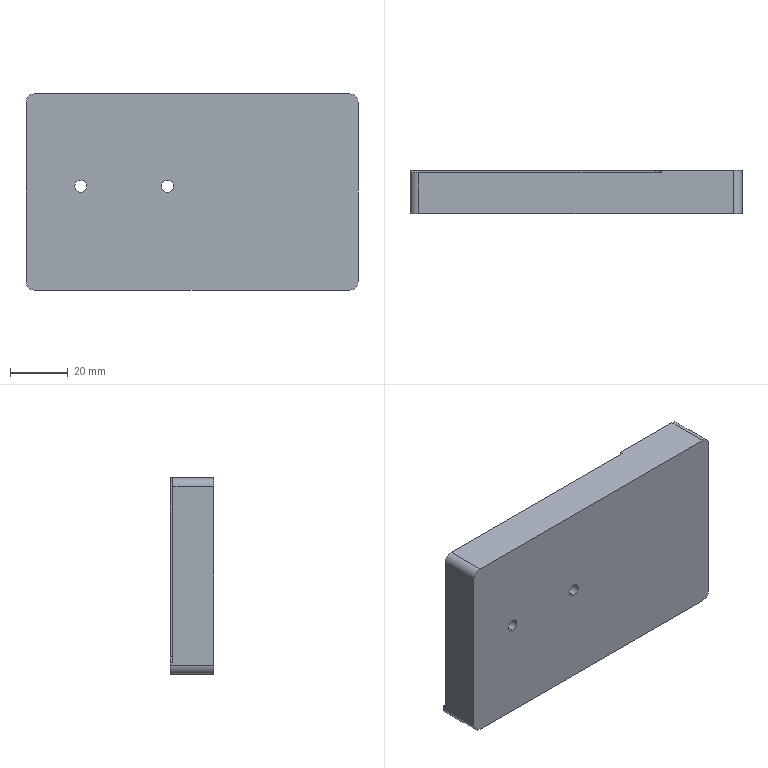Part | STEP file | 10000020445swp000-1 | 1 solid | 26 faces | box 115 x 15 x 68 mm | volume 111374 mm3 | cylinder 13 | plane 9 | cone 4 | commonest cylinder face diameters 4.2 x8 6 x4 4 x1
STEP:
#1=CARTESIAN_POINT('',(7.1,7.5,-19.6));
#2=VERTEX_POINT('',#1);
#3=CARTESIAN_POINT('',(2.9,7.5,-19.6));
#4=VERTEX_POINT('',#3);
#5=CARTESIAN_POINT('',(5.,7.5,-19.6));
#6=DIRECTION('',(0.,0.,-1.));
#7=DIRECTION('',(-1.,0.,0.));
#8=AXIS2_PLACEMENT_3D('',#5,#6,#7);
#9=CIRCLE('',#8,2.1);
#10=EDGE_CURVE('',#2,#4,#9,.T.);
#11=ORIENTED_EDGE('',*,*,#10,.F.);
#12=CARTESIAN_POINT('',(7.1,7.5,-34.));
#13=VERTEX_POINT('',#12);
#14=CARTESIAN_POINT('',(7.1,7.5,-34.));
#15=DIRECTION('',(0.,0.,-1.));
#16=VECTOR('',#15,1000.);
#17=LINE('',#14,#16);
#18=EDGE_CURVE('',#2,#13,#17,.T.);
#19=ORIENTED_EDGE('',*,*,#18,.T.);
#20=CARTESIAN_POINT('',(2.9,7.5,-34.));
#21=VERTEX_POINT('',#20);
#22=CARTESIAN_POINT('',(5.,7.5,-34.));
#23=DIRECTION('',(0.,0.,-1.));
#24=DIRECTION('',(-1.,0.,0.));
#25=AXIS2_PLACEMENT_3D('',#22,#23,#24);
#26=CIRCLE('',#25,2.1);
#27=EDGE_CURVE('',#13,#21,#26,.T.);
#28=ORIENTED_EDGE('',*,*,#27,.T.);
#29=CARTESIAN_POINT('',(2.9,7.5,-34.));
#30=DIRECTION('',(0.,0.,-1.));
#31=VECTOR('',#30,1000.);
#32=LINE('',#29,#31);
#33=EDGE_CURVE('',#4,#21,#32,.T.);
#34=ORIENTED_EDGE('',*,*,#33,.F.);
#35=EDGE_LOOP('',(#11,#19,#28,#34));
#36=FACE_OUTER_BOUND('',#35,.T.);
#37=CARTESIAN_POINT('',(5.,7.5,-34.));
#38=DIRECTION('',(0.,0.,-1.));
#39=DIRECTION('',(-1.,0.,0.));
#40=AXIS2_PLACEMENT_3D('',#37,#38,#39);
#41=CYLINDRICAL_SURFACE('',#40,2.1);
#42=ADVANCED_FACE('',(#36),#41,.F.);
#43=CARTESIAN_POINT('',(5.,7.5,-18.338));
#44=VERTEX_POINT('',#43);
#45=CARTESIAN_POINT('',(2.9,7.5,-19.6));
#46=DIRECTION('',(-0.8572,0.,-0.515));
#47=VECTOR('',#46,1000.);
#48=LINE('',#45,#47);
#49=EDGE_CURVE('',#44,#4,#48,.T.);
#50=ORIENTED_EDGE('',*,*,#49,.F.);
#51=CARTESIAN_POINT('',(7.1,7.5,-19.6));
#52=DIRECTION('',(0.8572,0.,-0.515));
#53=VECTOR('',#52,1000.);
#54=LINE('',#51,#53);
#55=EDGE_CURVE('',#44,#2,#54,.T.);
#56=ORIENTED_EDGE('',*,*,#55,.T.);
#57=ORIENTED_EDGE('',*,*,#10,.T.);
#58=EDGE_LOOP('',(#50,#56,#57));
#59=FACE_OUTER_BOUND('',#58,.T.);
#60=CARTESIAN_POINT('',(5.,7.5,-19.6));
#61=DIRECTION('',(0.,0.,-1.));
#62=DIRECTION('',(-1.,0.,0.));
#63=AXIS2_PLACEMENT_3D('',#60,#61,#62);
#64=CONICAL_SURFACE('',#63,2.1,1.03);
#65=ADVANCED_FACE('',(#59),#64,.F.);
#66=CARTESIAN_POINT('',(-38.9,7.5,-19.6));
#67=VERTEX_POINT('',#66);
#68=CARTESIAN_POINT('',(-43.1,7.5,-19.6));
#69=VERTEX_POINT('',#68);
#70=CARTESIAN_POINT('',(-41.,7.5,-19.6));
#71=DIRECTION('',(0.,0.,-1.));
#72=DIRECTION('',(-1.,0.,0.));
#73=AXIS2_PLACEMENT_3D('',#70,#71,#72);
#74=CIRCLE('',#73,2.1);
#75=EDGE_CURVE('',#67,#69,#74,.T.);
#76=ORIENTED_EDGE('',*,*,#75,.F.);
#77=CARTESIAN_POINT('',(-38.9,7.5,-34.));
#78=VERTEX_POINT('',#77);
#79=CARTESIAN_POINT('',(-38.9,7.5,-34.));
#80=DIRECTION('',(0.,0.,-1.));
#81=VECTOR('',#80,1000.);
#82=LINE('',#79,#81);
#83=EDGE_CURVE('',#67,#78,#82,.T.);
#84=ORIENTED_EDGE('',*,*,#83,.T.);
#85=CARTESIAN_POINT('',(-43.1,7.5,-34.));
#86=VERTEX_POINT('',#85);
#87=CARTESIAN_POINT('',(-41.,7.5,-34.));
#88=DIRECTION('',(0.,0.,-1.));
#89=DIRECTION('',(-1.,0.,0.));
#90=AXIS2_PLACEMENT_3D('',#87,#88,#89);
#91=CIRCLE('',#90,2.1);
#92=EDGE_CURVE('',#78,#86,#91,.T.);
#93=ORIENTED_EDGE('',*,*,#92,.T.);
#94=CARTESIAN_POINT('',(-43.1,7.5,-34.));
#95=DIRECTION('',(0.,0.,-1.));
#96=VECTOR('',#95,1000.);
#97=LINE('',#94,#96);
#98=EDGE_CURVE('',#69,#86,#97,.T.);
#99=ORIENTED_EDGE('',*,*,#98,.F.);
#100=EDGE_LOOP('',(#76,#84,#93,#99));
#101=FACE_OUTER_BOUND('',#100,.T.);
#102=CARTESIAN_POINT('',(-41.,7.5,-34.));
#103=DIRECTION('',(0.,0.,-1.));
#104=DIRECTION('',(-1.,0.,0.));
#105=AXIS2_PLACEMENT_3D('',#102,#103,#104);
#106=CYLINDRICAL_SURFACE('',#105,2.1);
#107=ADVANCED_FACE('',(#101),#106,.F.);
#108=CARTESIAN_POINT('',(-41.,7.5,-18.338));
#109=VERTEX_POINT('',#108);
#110=CARTESIAN_POINT('',(-43.1,7.5,-19.6));
#111=DIRECTION('',(-0.8572,0.,-0.515));
#112=VECTOR('',#111,1000.);
#113=LINE('',#110,#112);
#114=EDGE_CURVE('',#109,#69,#113,.T.);
#115=ORIENTED_EDGE('',*,*,#114,.F.);
#116=CARTESIAN_POINT('',(-38.9,7.5,-19.6));
#117=DIRECTION('',(0.8572,0.,-0.515));
#118=VECTOR('',#117,1000.);
#119=LINE('',#116,#118);
#120=EDGE_CURVE('',#109,#67,#119,.T.);
#121=ORIENTED_EDGE('',*,*,#120,.T.);
#122=ORIENTED_EDGE('',*,*,#75,.T.);
#123=EDGE_LOOP('',(#115,#121,#122));
#124=FACE_OUTER_BOUND('',#123,.T.);
#125=CARTESIAN_POINT('',(-41.,7.5,-19.6));
#126=DIRECTION('',(0.,0.,-1.));
#127=DIRECTION('',(-1.,0.,0.));
#128=AXIS2_PLACEMENT_3D('',#125,#126,#127);
#129=CONICAL_SURFACE('',#128,2.1,1.03);
#130=ADVANCED_FACE('',(#124),#129,.F.);
#131=CARTESIAN_POINT('',(-8.5,0.,-0.1));
#132=VERTEX_POINT('',#131);
#133=CARTESIAN_POINT('',(-8.5,0.,4.1));
#134=VERTEX_POINT('',#133);
#135=CARTESIAN_POINT('',(-8.5,0.,2.));
#136=DIRECTION('',(0.,1.,0.));
#137=DIRECTION('',(0.,0.,1.));
#138=AXIS2_PLACEMENT_3D('',#135,#136,#137);
#139=CIRCLE('',#138,2.1);
#140=EDGE_CURVE('',#132,#134,#139,.T.);
#141=ORIENTED_EDGE('',*,*,#140,.F.);
#142=CARTESIAN_POINT('',(-8.5,14.1,-0.1));
#143=VERTEX_POINT('',#142);
#144=CARTESIAN_POINT('',(-8.5,14.1,-0.1));
#145=DIRECTION('',(0.,1.,0.));
#146=VECTOR('',#145,1000.);
#147=LINE('',#144,#146);
#148=EDGE_CURVE('',#132,#143,#147,.T.);
#149=ORIENTED_EDGE('',*,*,#148,.T.);
#150=CARTESIAN_POINT('',(-8.5,14.1,4.1));
#151=VERTEX_POINT('',#150);
#152=CARTESIAN_POINT('',(-8.5,14.1,2.));
#153=DIRECTION('',(0.,1.,0.));
#154=DIRECTION('',(0.,0.,1.));
#155=AXIS2_PLACEMENT_3D('',#152,#153,#154);
#156=CIRCLE('',#155,2.1);
#157=EDGE_CURVE('',#143,#151,#156,.T.);
#158=ORIENTED_EDGE('',*,*,#157,.T.);
#159=CARTESIAN_POINT('',(-8.5,14.1,4.1));
#160=DIRECTION('',(0.,1.,0.));
#161=VECTOR('',#160,1000.);
#162=LINE('',#159,#161);
#163=EDGE_CURVE('',#134,#151,#162,.T.);
#164=ORIENTED_EDGE('',*,*,#163,.F.);
#165=EDGE_LOOP('',(#141,#149,#158,#164));
#166=FACE_OUTER_BOUND('',#165,.T.);
#167=CARTESIAN_POINT('',(-8.5,14.1,2.));
#168=DIRECTION('',(0.,1.,0.));
#169=DIRECTION('',(0.,0.,1.));
#170=AXIS2_PLACEMENT_3D('',#167,#168,#169);
#171=CYLINDRICAL_SURFACE('',#170,2.1);
#172=ADVANCED_FACE('',(#166),#171,.F.);
#173=CARTESIAN_POINT('',(-38.5,0.,-0.1));
#174=VERTEX_POINT('',#173);
#175=CARTESIAN_POINT('',(-38.5,0.,4.1));
#176=VERTEX_POINT('',#175);
#177=CARTESIAN_POINT('',(-38.5,0.,2.));
#178=DIRECTION('',(0.,1.,0.));
#179=DIRECTION('',(0.,0.,1.));
#180=AXIS2_PLACEMENT_3D('',#177,#178,#179);
#181=CIRCLE('',#180,2.1);
#182=EDGE_CURVE('',#174,#176,#181,.T.);
#183=ORIENTED_EDGE('',*,*,#182,.F.);
#184=CARTESIAN_POINT('',(-38.5,14.1,-0.1));
#185=VERTEX_POINT('',#184);
#186=CARTESIAN_POINT('',(-38.5,14.1,-0.1));
#187=DIRECTION('',(0.,1.,0.));
#188=VECTOR('',#187,1000.);
#189=LINE('',#186,#188);
#190=EDGE_CURVE('',#174,#185,#189,.T.);
#191=ORIENTED_EDGE('',*,*,#190,.T.);
#192=CARTESIAN_POINT('',(-38.5,14.1,4.1));
#193=VERTEX_POINT('',#192);
#194=CARTESIAN_POINT('',(-38.5,14.1,2.));
#195=DIRECTION('',(0.,1.,0.));
#196=DIRECTION('',(0.,0.,1.));
#197=AXIS2_PLACEMENT_3D('',#194,#195,#196);
#198=CIRCLE('',#197,2.1);
#199=EDGE_CURVE('',#185,#193,#198,.T.);
#200=ORIENTED_EDGE('',*,*,#199,.T.);
#201=CARTESIAN_POINT('',(-38.5,14.1,4.1));
#202=DIRECTION('',(0.,1.,0.));
#203=VECTOR('',#202,1000.);
#204=LINE('',#201,#203);
#205=EDGE_CURVE('',#176,#193,#204,.T.);
#206=ORIENTED_EDGE('',*,*,#205,.F.);
#207=EDGE_LOOP('',(#183,#191,#200,#206));
#208=FACE_OUTER_BOUND('',#207,.T.);
#209=CARTESIAN_POINT('',(-38.5,14.1,2.));
#210=DIRECTION('',(0.,1.,0.));
#211=DIRECTION('',(0.,0.,1.));
#212=AXIS2_PLACEMENT_3D('',#209,#210,#211);
#213=CYLINDRICAL_SURFACE('',#212,2.1);
#214=ADVANCED_FACE('',(#208),#213,.F.);
#215=CARTESIAN_POINT('',(57.5,0.,31.));
#216=VERTEX_POINT('',#215);
#217=CARTESIAN_POINT('',(57.5,0.,-31.));
#218=VERTEX_POINT('',#217);
#219=CARTESIAN_POINT('',(57.5,0.,-34.));
#220=DIRECTION('',(0.,0.,-1.));
#221=VECTOR('',#220,1000.);
#222=LINE('',#219,#221);
#223=EDGE_CURVE('',#216,#218,#222,.T.);
#224=ORIENTED_EDGE('',*,*,#223,.T.);
#225=CARTESIAN_POINT('',(57.5,15.,-31.));
#226=VERTEX_POINT('',#225);
#227=CARTESIAN_POINT('',(57.5,15.,-31.));
#228=DIRECTION('',(0.,1.,0.));
#229=VECTOR('',#228,1000.);
#230=LINE('',#227,#229);
#231=EDGE_CURVE('',#218,#226,#230,.T.);
#232=ORIENTED_EDGE('',*,*,#231,.T.);
#233=CARTESIAN_POINT('',(57.5,15.,31.));
#234=VERTEX_POINT('',#233);
#235=CARTESIAN_POINT('',(57.5,15.,-34.));
#236=DIRECTION('',(0.,0.,-1.));
#237=VECTOR('',#236,1000.);
#238=LINE('',#235,#237);
#239=EDGE_CURVE('',#234,#226,#238,.T.);
#240=ORIENTED_EDGE('',*,*,#239,.F.);
#241=CARTESIAN_POINT('',(57.5,15.,31.));
#242=DIRECTION('',(0.,-1.,0.));
#243=VECTOR('',#242,1000.);
#244=LINE('',#241,#243);
#245=EDGE_CURVE('',#234,#216,#244,.T.);
#246=ORIENTED_EDGE('',*,*,#245,.T.);
#247=EDGE_LOOP('',(#224,#232,#240,#246));
#248=FACE_OUTER_BOUND('',#247,.T.);
#249=CARTESIAN_POINT('',(57.5,15.,-34.));
#250=DIRECTION('',(-1.,0.,0.));
#251=DIRECTION('',(0.,0.,1.));
#252=AXIS2_PLACEMENT_3D('',#249,#250,#251);
#253=PLANE('',#252);
#254=ADVANCED_FACE('',(#248),#253,.F.);
#255=CARTESIAN_POINT('',(5.,7.5,-34.));
#256=DIRECTION('',(0.,0.,-1.));
#257=DIRECTION('',(-1.,0.,0.));
#258=AXIS2_PLACEMENT_3D('',#255,#256,#257);
#259=CIRCLE('',#258,2.1);
#260=EDGE_CURVE('',#21,#13,#259,.T.);
#261=ORIENTED_EDGE('',*,*,#260,.F.);
#262=ORIENTED_EDGE('',*,*,#27,.F.);
#263=EDGE_LOOP('',(#261,#262));
#264=FACE_BOUND('',#263,.T.);
#265=CARTESIAN_POINT('',(-41.,7.5,-34.));
#266=DIRECTION('',(0.,0.,-1.));
#267=DIRECTION('',(-1.,0.,0.));
#268=AXIS2_PLACEMENT_3D('',#265,#266,#267);
#269=CIRCLE('',#268,2.1);
#270=EDGE_CURVE('',#86,#78,#269,.T.);
#271=ORIENTED_EDGE('',*,*,#270,.F.);
#272=ORIENTED_EDGE('',*,*,#92,.F.);
#273=EDGE_LOOP('',(#271,#272));
#274=FACE_BOUND('',#273,.T.);
#275=CARTESIAN_POINT('',(54.5,15.,-34.));
#276=VERTEX_POINT('',#275);
#277=CARTESIAN_POINT('',(-54.5,15.,-34.));
#278=VERTEX_POINT('',#277);
#279=CARTESIAN_POINT('',(-57.5,15.,-34.));
#280=DIRECTION('',(-1.,0.,0.));
#281=VECTOR('',#280,1000.);
#282=LINE('',#279,#281);
#283=EDGE_CURVE('',#276,#278,#282,.T.);
#284=ORIENTED_EDGE('',*,*,#283,.F.);
#285=CARTESIAN_POINT('',(54.5,0.,-34.));
#286=VERTEX_POINT('',#285);
#287=CARTESIAN_POINT('',(54.5,15.,-34.));
#288=DIRECTION('',(0.,-1.,0.));
#289=VECTOR('',#288,1000.);
#290=LINE('',#287,#289);
#291=EDGE_CURVE('',#276,#286,#290,.T.);
#292=ORIENTED_EDGE('',*,*,#291,.T.);
#293=CARTESIAN_POINT('',(-54.5,0.,-34.));
#294=VERTEX_POINT('',#293);
#295=CARTESIAN_POINT('',(-57.5,0.,-34.));
#296=DIRECTION('',(-1.,0.,0.));
#297=VECTOR('',#296,1000.);
#298=LINE('',#295,#297);
#299=EDGE_CURVE('',#286,#294,#298,.T.);
#300=ORIENTED_EDGE('',*,*,#299,.T.);
#301=CARTESIAN_POINT('',(-54.5,15.,-34.));
#302=DIRECTION('',(0.,1.,0.));
#303=VECTOR('',#302,1000.);
#304=LINE('',#301,#303);
#305=EDGE_CURVE('',#294,#278,#304,.T.);
#306=ORIENTED_EDGE('',*,*,#305,.T.);
#307=EDGE_LOOP('',(#284,#292,#300,#306));
#308=FACE_OUTER_BOUND('',#307,.T.);
#309=CARTESIAN_POINT('',(-57.5,15.,-34.));
#310=DIRECTION('',(0.,0.,1.));
#311=DIRECTION('',(1.,0.,0.));
#312=AXIS2_PLACEMENT_3D('',#309,#310,#311);
#313=PLANE('',#312);
#314=ADVANCED_FACE('',(#264,#274,#308),#313,.F.);
#315=CARTESIAN_POINT('',(-57.5,15.,-31.));
#316=VERTEX_POINT('',#315);
#317=CARTESIAN_POINT('',(-57.5,15.,-30.));
#318=VERTEX_POINT('',#317);
#319=CARTESIAN_POINT('',(-57.5,15.,-34.));
#320=DIRECTION('',(0.,0.,1.));
#321=VECTOR('',#320,1000.);
#322=LINE('',#319,#321);
#323=EDGE_CURVE('',#316,#318,#322,.T.);
#324=ORIENTED_EDGE('',*,*,#323,.F.);
#325=CARTESIAN_POINT('',(-57.5,0.,-31.));
#326=VERTEX_POINT('',#325);
#327=CARTESIAN_POINT('',(-57.5,15.,-31.));
#328=DIRECTION('',(0.,-1.,0.));
#329=VECTOR('',#328,1000.);
#330=LINE('',#327,#329);
#331=EDGE_CURVE('',#316,#326,#330,.T.);
#332=ORIENTED_EDGE('',*,*,#331,.T.);
#333=CARTESIAN_POINT('',(-57.5,0.,31.));
#334=VERTEX_POINT('',#333);
#335=CARTESIAN_POINT('',(-57.5,0.,-34.));
#336=DIRECTION('',(0.,0.,1.));
#337=VECTOR('',#336,1000.);
#338=LINE('',#335,#337);
#339=EDGE_CURVE('',#326,#334,#338,.T.);
#340=ORIENTED_EDGE('',*,*,#339,.T.);
#341=CARTESIAN_POINT('',(-57.5,14.1,31.));
#342=VERTEX_POINT('',#341);
#343=CARTESIAN_POINT('',(-57.5,15.,31.));
#344=DIRECTION('',(0.,1.,0.));
#345=VECTOR('',#344,1000.);
#346=LINE('',#343,#345);
#347=EDGE_CURVE('',#334,#342,#346,.T.);
#348=ORIENTED_EDGE('',*,*,#347,.T.);
#349=CARTESIAN_POINT('',(-57.5,14.1,-30.));
#350=VERTEX_POINT('',#349);
#351=CARTESIAN_POINT('',(-57.5,14.1,34.));
#352=DIRECTION('',(0.,0.,1.));
#353=VECTOR('',#352,1000.);
#354=LINE('',#351,#353);
#355=EDGE_CURVE('',#350,#342,#354,.T.);
#356=ORIENTED_EDGE('',*,*,#355,.F.);
#357=CARTESIAN_POINT('',(-57.5,14.1,-30.));
#358=DIRECTION('',(0.,1.,0.));
#359=VECTOR('',#358,1000.);
#360=LINE('',#357,#359);
#361=EDGE_CURVE('',#350,#318,#360,.T.);
#362=ORIENTED_EDGE('',*,*,#361,.T.);
#363=EDGE_LOOP('',(#324,#332,#340,#348,#356,#362));
#364=FACE_OUTER_BOUND('',#363,.T.);
#365=CARTESIAN_POINT('',(-57.5,15.,-34.));
#366=DIRECTION('',(1.,0.,0.));
#367=DIRECTION('',(0.,0.,-1.));
#368=AXIS2_PLACEMENT_3D('',#365,#366,#367);
#369=PLANE('',#368);
#370=ADVANCED_FACE('',(#364),#369,.F.);
#371=CARTESIAN_POINT('',(-54.5,14.1,34.));
#372=VERTEX_POINT('',#371);
#373=CARTESIAN_POINT('',(29.5,14.1,34.));
#374=VERTEX_POINT('',#373);
#375=CARTESIAN_POINT('',(29.5,14.1,34.));
#376=DIRECTION('',(1.,0.,0.));
#377=VECTOR('',#376,1000.);
#378=LINE('',#375,#377);
#379=EDGE_CURVE('',#372,#374,#378,.T.);
#380=ORIENTED_EDGE('',*,*,#379,.F.);
#381=CARTESIAN_POINT('',(-54.5,0.,34.));
#382=VERTEX_POINT('',#381);
#383=CARTESIAN_POINT('',(-54.5,15.,34.));
#384=DIRECTION('',(0.,-1.,0.));
#385=VECTOR('',#384,1000.);
#386=LINE('',#383,#385);
#387=EDGE_CURVE('',#372,#382,#386,.T.);
#388=ORIENTED_EDGE('',*,*,#387,.T.);
#389=CARTESIAN_POINT('',(54.5,0.,34.));
#390=VERTEX_POINT('',#389);
#391=CARTESIAN_POINT('',(-57.5,0.,34.));
#392=DIRECTION('',(1.,0.,0.));
#393=VECTOR('',#392,1000.);
#394=LINE('',#391,#393);
#395=EDGE_CURVE('',#382,#390,#394,.T.);
#396=ORIENTED_EDGE('',*,*,#395,.T.);
#397=CARTESIAN_POINT('',(54.5,15.,34.));
#398=VERTEX_POINT('',#397);
#399=CARTESIAN_POINT('',(54.5,15.,34.));
#400=DIRECTION('',(0.,1.,0.));
#401=VECTOR('',#400,1000.);
#402=LINE('',#399,#401);
#403=EDGE_CURVE('',#390,#398,#402,.T.);
#404=ORIENTED_EDGE('',*,*,#403,.T.);
#405=CARTESIAN_POINT('',(29.5,15.,34.));
#406=VERTEX_POINT('',#405);
#407=CARTESIAN_POINT('',(-57.5,15.,34.));
#408=DIRECTION('',(1.,0.,0.));
#409=VECTOR('',#408,1000.);
#410=LINE('',#407,#409);
#411=EDGE_CURVE('',#406,#398,#410,.T.);
#412=ORIENTED_EDGE('',*,*,#411,.F.);
#413=CARTESIAN_POINT('',(29.5,14.1,34.));
#414=DIRECTION('',(0.,1.,0.));
#415=VECTOR('',#414,1000.);
#416=LINE('',#413,#415);
#417=EDGE_CURVE('',#374,#406,#416,.T.);
#418=ORIENTED_EDGE('',*,*,#417,.F.);
#419=EDGE_LOOP('',(#380,#388,#396,#404,#412,#418));
#420=FACE_OUTER_BOUND('',#419,.T.);
#421=CARTESIAN_POINT('',(-57.5,15.,34.));
#422=DIRECTION('',(0.,0.,-1.));
#423=DIRECTION('',(-1.,0.,0.));
#424=AXIS2_PLACEMENT_3D('',#421,#422,#423);
#425=PLANE('',#424);
#426=ADVANCED_FACE('',(#420),#425,.F.);
#427=ORIENTED_EDGE('',*,*,#239,.T.);
#428=CARTESIAN_POINT('',(54.5,15.,-31.));
#429=DIRECTION('',(0.,1.,0.));
#430=DIRECTION('',(0.,0.,1.));
#431=AXIS2_PLACEMENT_3D('',#428,#429,#430);
#432=CIRCLE('',#431,3.);
#433=EDGE_CURVE('',#226,#276,#432,.T.);
#434=ORIENTED_EDGE('',*,*,#433,.T.);
#435=ORIENTED_EDGE('',*,*,#283,.T.);
#436=CARTESIAN_POINT('',(-54.5,15.,-31.));
#437=DIRECTION('',(0.,1.,0.));
#438=DIRECTION('',(0.,0.,1.));
#439=AXIS2_PLACEMENT_3D('',#436,#437,#438);
#440=CIRCLE('',#439,3.);
#441=EDGE_CURVE('',#278,#316,#440,.T.);
#442=ORIENTED_EDGE('',*,*,#441,.T.);
#443=ORIENTED_EDGE('',*,*,#323,.T.);
#444=CARTESIAN_POINT('',(27.5,15.,-30.));
#445=VERTEX_POINT('',#444);
#446=CARTESIAN_POINT('',(29.5,15.,-30.));
#447=DIRECTION('',(-1.,0.,0.));
#448=VECTOR('',#447,1000.);
#449=LINE('',#446,#448);
#450=EDGE_CURVE('',#445,#318,#449,.T.);
#451=ORIENTED_EDGE('',*,*,#450,.F.);
#452=CARTESIAN_POINT('',(29.5,15.,-28.));
#453=VERTEX_POINT('',#452);
#454=CARTESIAN_POINT('',(27.5,15.,-28.));
#455=DIRECTION('',(0.,-1.,0.));
#456=DIRECTION('',(0.,0.,1.));
#457=AXIS2_PLACEMENT_3D('',#454,#455,#456);
#458=CIRCLE('',#457,2.);
#459=EDGE_CURVE('',#445,#453,#458,.T.);
#460=ORIENTED_EDGE('',*,*,#459,.T.);
#461=CARTESIAN_POINT('',(29.5,15.,34.));
#462=DIRECTION('',(0.,0.,-1.));
#463=VECTOR('',#462,1000.);
#464=LINE('',#461,#463);
#465=EDGE_CURVE('',#406,#453,#464,.T.);
#466=ORIENTED_EDGE('',*,*,#465,.F.);
#467=ORIENTED_EDGE('',*,*,#411,.T.);
#468=CARTESIAN_POINT('',(54.5,15.,31.));
#469=DIRECTION('',(0.,1.,0.));
#470=DIRECTION('',(0.,0.,1.));
#471=AXIS2_PLACEMENT_3D('',#468,#469,#470);
#472=CIRCLE('',#471,3.);
#473=EDGE_CURVE('',#398,#234,#472,.T.);
#474=ORIENTED_EDGE('',*,*,#473,.T.);
#475=EDGE_LOOP('',(#427,#434,#435,#442,#443,#451,#460,#466,#467,#474));
#476=FACE_OUTER_BOUND('',#475,.T.);
#477=CARTESIAN_POINT('',(0.,15.,0.));
#478=DIRECTION('',(0.,1.,0.));
#479=DIRECTION('',(0.,0.,1.));
#480=AXIS2_PLACEMENT_3D('',#477,#478,#479);
#481=PLANE('',#480);
#482=ADVANCED_FACE('',(#476),#481,.T.);
#483=CARTESIAN_POINT('',(-8.5,0.,2.));
#484=DIRECTION('',(0.,1.,0.));
#485=DIRECTION('',(0.,0.,1.));
#486=AXIS2_PLACEMENT_3D('',#483,#484,#485);
#487=CIRCLE('',#486,2.1);
#488=EDGE_CURVE('',#134,#132,#487,.T.);
#489=ORIENTED_EDGE('',*,*,#488,.T.);
#490=ORIENTED_EDGE('',*,*,#140,.T.);
#491=EDGE_LOOP('',(#489,#490));
#492=FACE_BOUND('',#491,.T.);
#493=CARTESIAN_POINT('',(-38.5,0.,2.));
#494=DIRECTION('',(0.,1.,0.));
#495=DIRECTION('',(0.,0.,1.));
#496=AXIS2_PLACEMENT_3D('',#493,#494,#495);
#497=CIRCLE('',#496,2.1);
#498=EDGE_CURVE('',#176,#174,#497,.T.);
#499=ORIENTED_EDGE('',*,*,#498,.T.);
#500=ORIENTED_EDGE('',*,*,#182,.T.);
#501=EDGE_LOOP('',(#499,#500));
#502=FACE_BOUND('',#501,.T.);
#503=ORIENTED_EDGE('',*,*,#299,.F.);
#504=CARTESIAN_POINT('',(54.5,0.,-31.));
#505=DIRECTION('',(0.,-1.,0.));
#506=DIRECTION('',(0.,0.,1.));
#507=AXIS2_PLACEMENT_3D('',#504,#505,#506);
#508=CIRCLE('',#507,3.);
#509=EDGE_CURVE('',#286,#218,#508,.T.);
#510=ORIENTED_EDGE('',*,*,#509,.T.);
#511=ORIENTED_EDGE('',*,*,#223,.F.);
#512=CARTESIAN_POINT('',(54.5,0.,31.));
#513=DIRECTION('',(0.,-1.,0.));
#514=DIRECTION('',(0.,0.,1.));
#515=AXIS2_PLACEMENT_3D('',#512,#513,#514);
#516=CIRCLE('',#515,3.);
#517=EDGE_CURVE('',#216,#390,#516,.T.);
#518=ORIENTED_EDGE('',*,*,#517,.T.);
#519=ORIENTED_EDGE('',*,*,#395,.F.);
#520=CARTESIAN_POINT('',(-54.5,0.,31.));
#521=DIRECTION('',(0.,-1.,0.));
#522=DIRECTION('',(0.,0.,1.));
#523=AXIS2_PLACEMENT_3D('',#520,#521,#522);
#524=CIRCLE('',#523,3.);
#525=EDGE_CURVE('',#382,#334,#524,.T.);
#526=ORIENTED_EDGE('',*,*,#525,.T.);
#527=ORIENTED_EDGE('',*,*,#339,.F.);
#528=CARTESIAN_POINT('',(-54.5,0.,-31.));
#529=DIRECTION('',(0.,-1.,0.));
#530=DIRECTION('',(0.,0.,1.));
#531=AXIS2_PLACEMENT_3D('',#528,#529,#530);
#532=CIRCLE('',#531,3.);
#533=EDGE_CURVE('',#326,#294,#532,.T.);
#534=ORIENTED_EDGE('',*,*,#533,.T.);
#535=EDGE_LOOP('',(#503,#510,#511,#518,#519,#526,#527,#534));
#536=FACE_OUTER_BOUND('',#535,.T.);
#537=CARTESIAN_POINT('',(0.,0.,0.));
#538=DIRECTION('',(0.,1.,0.));
#539=DIRECTION('',(0.,0.,1.));
#540=AXIS2_PLACEMENT_3D('',#537,#538,#539);
#541=PLANE('',#540);
#542=ADVANCED_FACE('',(#492,#502,#536),#541,.F.);
#543=ORIENTED_EDGE('',*,*,#465,.T.);
#544=CARTESIAN_POINT('',(29.5,14.1,-28.));
#545=VERTEX_POINT('',#544);
#546=CARTESIAN_POINT('',(29.5,14.1,-28.));
#547=DIRECTION('',(0.,-1.,0.));
#548=VECTOR('',#547,1000.);
#549=LINE('',#546,#548);
#550=EDGE_CURVE('',#453,#545,#549,.T.);
#551=ORIENTED_EDGE('',*,*,#550,.T.);
#552=CARTESIAN_POINT('',(29.5,14.1,34.));
#553=DIRECTION('',(0.,0.,-1.));
#554=VECTOR('',#553,1000.);
#555=LINE('',#552,#554);
#556=EDGE_CURVE('',#374,#545,#555,.T.);
#557=ORIENTED_EDGE('',*,*,#556,.F.);
#558=ORIENTED_EDGE('',*,*,#417,.T.);
#559=EDGE_LOOP('',(#543,#551,#557,#558));
#560=FACE_OUTER_BOUND('',#559,.T.);
#561=CARTESIAN_POINT('',(29.5,14.1,34.));
#562=DIRECTION('',(1.,0.,0.));
#563=DIRECTION('',(0.,0.,-1.));
#564=AXIS2_PLACEMENT_3D('',#561,#562,#563);
#565=PLANE('',#564);
#566=ADVANCED_FACE('',(#560),#565,.F.);
#567=CARTESIAN_POINT('',(27.5,14.1,-30.));
#568=VERTEX_POINT('',#567);
#569=CARTESIAN_POINT('',(29.5,14.1,-30.));
#570=DIRECTION('',(-1.,0.,0.));
#571=VECTOR('',#570,1000.);
#572=LINE('',#569,#571);
#573=EDGE_CURVE('',#568,#350,#572,.T.);
#574=ORIENTED_EDGE('',*,*,#573,.F.);
#575=CARTESIAN_POINT('',(27.5,15.,-30.));
#576=DIRECTION('',(0.,1.,0.));
#577=VECTOR('',#576,1000.);
#578=LINE('',#575,#577);
#579=EDGE_CURVE('',#568,#445,#578,.T.);
#580=ORIENTED_EDGE('',*,*,#579,.T.);
#581=ORIENTED_EDGE('',*,*,#450,.T.);
#582=ORIENTED_EDGE('',*,*,#361,.F.);
#583=EDGE_LOOP('',(#574,#580,#581,#582));
#584=FACE_OUTER_BOUND('',#583,.T.);
#585=CARTESIAN_POINT('',(29.5,14.1,-30.));
#586=DIRECTION('',(0.,0.,-1.));
#587=DIRECTION('',(-1.,0.,0.));
#588=AXIS2_PLACEMENT_3D('',#585,#586,#587);
#589=PLANE('',#588);
#590=ADVANCED_FACE('',(#584),#589,.F.);
#591=CARTESIAN_POINT('',(-8.5,14.1,2.));
#592=DIRECTION('',(0.,1.,0.));
#593=DIRECTION('',(0.,0.,1.));
#594=AXIS2_PLACEMENT_3D('',#591,#592,#593);
#595=CIRCLE('',#594,2.1);
#596=EDGE_CURVE('',#151,#143,#595,.T.);
#597=ORIENTED_EDGE('',*,*,#596,.F.);
#598=ORIENTED_EDGE('',*,*,#157,.F.);
#599=EDGE_LOOP('',(#597,#598));
#600=FACE_BOUND('',#599,.T.);
#601=CARTESIAN_POINT('',(-38.5,14.1,2.));
#602=DIRECTION('',(0.,1.,0.));
#603=DIRECTION('',(0.,0.,1.));
#604=AXIS2_PLACEMENT_3D('',#601,#602,#603);
#605=CIRCLE('',#604,2.1);
#606=EDGE_CURVE('',#193,#185,#605,.T.);
#607=ORIENTED_EDGE('',*,*,#606,.F.);
#608=ORIENTED_EDGE('',*,*,#199,.F.);
#609=EDGE_LOOP('',(#607,#608));
#610=FACE_BOUND('',#609,.T.);
#611=ORIENTED_EDGE('',*,*,#556,.T.);
#612=CARTESIAN_POINT('',(27.5,14.1,-28.));
#613=DIRECTION('',(0.,1.,0.));
#614=DIRECTION('',(0.,0.,1.));
#615=AXIS2_PLACEMENT_3D('',#612,#613,#614);
#616=CIRCLE('',#615,2.);
#617=EDGE_CURVE('',#545,#568,#616,.T.);
#618=ORIENTED_EDGE('',*,*,#617,.T.);
#619=ORIENTED_EDGE('',*,*,#573,.T.);
#620=ORIENTED_EDGE('',*,*,#355,.T.);
#621=CARTESIAN_POINT('',(-54.5,14.1,31.));
#622=DIRECTION('',(0.,1.,0.));
#623=DIRECTION('',(0.,0.,1.));
#624=AXIS2_PLACEMENT_3D('',#621,#622,#623);
#625=CIRCLE('',#624,3.);
#626=EDGE_CURVE('',#342,#372,#625,.T.);
#627=ORIENTED_EDGE('',*,*,#626,.T.);
#628=ORIENTED_EDGE('',*,*,#379,.T.);
#629=EDGE_LOOP('',(#611,#618,#619,#620,#627,#628));
#630=FACE_OUTER_BOUND('',#629,.T.);
#631=CARTESIAN_POINT('',(0.,14.1,0.));
#632=DIRECTION('',(0.,1.,0.));
#633=DIRECTION('',(0.,0.,1.));
#634=AXIS2_PLACEMENT_3D('',#631,#632,#633);
#635=PLANE('',#634);
#636=ADVANCED_FACE('',(#600,#610,#630),#635,.T.);
#637=ORIENTED_EDGE('',*,*,#190,.F.);
#638=ORIENTED_EDGE('',*,*,#498,.F.);
#639=ORIENTED_EDGE('',*,*,#205,.T.);
#640=ORIENTED_EDGE('',*,*,#606,.T.);
#641=EDGE_LOOP('',(#637,#638,#639,#640));
#642=FACE_OUTER_BOUND('',#641,.T.);
#643=CARTESIAN_POINT('',(-38.5,14.1,2.));
#644=DIRECTION('',(0.,1.,0.));
#645=DIRECTION('',(0.,0.,1.));
#646=AXIS2_PLACEMENT_3D('',#643,#644,#645);
#647=CYLINDRICAL_SURFACE('',#646,2.1);
#648=ADVANCED_FACE('',(#642),#647,.F.);
#649=ORIENTED_EDGE('',*,*,#148,.F.);
#650=ORIENTED_EDGE('',*,*,#488,.F.);
#651=ORIENTED_EDGE('',*,*,#163,.T.);
#652=ORIENTED_EDGE('',*,*,#596,.T.);
#653=EDGE_LOOP('',(#649,#650,#651,#652));
#654=FACE_OUTER_BOUND('',#653,.T.);
#655=CARTESIAN_POINT('',(-8.5,14.1,2.));
#656=DIRECTION('',(0.,1.,0.));
#657=DIRECTION('',(0.,0.,1.));
#658=AXIS2_PLACEMENT_3D('',#655,#656,#657);
#659=CYLINDRICAL_SURFACE('',#658,2.1);
#660=ADVANCED_FACE('',(#654),#659,.F.);
#661=ORIENTED_EDGE('',*,*,#120,.F.);
#662=ORIENTED_EDGE('',*,*,#114,.T.);
#663=CARTESIAN_POINT('',(-41.,7.5,-19.6));
#664=DIRECTION('',(0.,0.,-1.));
#665=DIRECTION('',(-1.,0.,0.));
#666=AXIS2_PLACEMENT_3D('',#663,#664,#665);
#667=CIRCLE('',#666,2.1);
#668=EDGE_CURVE('',#69,#67,#667,.T.);
#669=ORIENTED_EDGE('',*,*,#668,.T.);
#670=EDGE_LOOP('',(#661,#662,#669));
#671=FACE_OUTER_BOUND('',#670,.T.);
#672=CARTESIAN_POINT('',(-41.,7.5,-19.6));
#673=DIRECTION('',(0.,0.,-1.));
#674=DIRECTION('',(-1.,0.,0.));
#675=AXIS2_PLACEMENT_3D('',#672,#673,#674);
#676=CONICAL_SURFACE('',#675,2.1,1.03);
#677=ADVANCED_FACE('',(#671),#676,.F.);
#678=ORIENTED_EDGE('',*,*,#83,.F.);
#679=ORIENTED_EDGE('',*,*,#668,.F.);
#680=ORIENTED_EDGE('',*,*,#98,.T.);
#681=ORIENTED_EDGE('',*,*,#270,.T.);
#682=EDGE_LOOP('',(#678,#679,#680,#681));
#683=FACE_OUTER_BOUND('',#682,.T.);
#684=CARTESIAN_POINT('',(-41.,7.5,-34.));
#685=DIRECTION('',(0.,0.,-1.));
#686=DIRECTION('',(-1.,0.,0.));
#687=AXIS2_PLACEMENT_3D('',#684,#685,#686);
#688=CYLINDRICAL_SURFACE('',#687,2.1);
#689=ADVANCED_FACE('',(#683),#688,.F.);
#690=ORIENTED_EDGE('',*,*,#55,.F.);
#691=ORIENTED_EDGE('',*,*,#49,.T.);
#692=CARTESIAN_POINT('',(5.,7.5,-19.6));
#693=DIRECTION('',(0.,0.,-1.));
#694=DIRECTION('',(-1.,0.,0.));
#695=AXIS2_PLACEMENT_3D('',#692,#693,#694);
#696=CIRCLE('',#695,2.1);
#697=EDGE_CURVE('',#4,#2,#696,.T.);
#698=ORIENTED_EDGE('',*,*,#697,.T.);
#699=EDGE_LOOP('',(#690,#691,#698));
#700=FACE_OUTER_BOUND('',#699,.T.);
#701=CARTESIAN_POINT('',(5.,7.5,-19.6));
#702=DIRECTION('',(0.,0.,-1.));
#703=DIRECTION('',(-1.,0.,0.));
#704=AXIS2_PLACEMENT_3D('',#701,#702,#703);
#705=CONICAL_SURFACE('',#704,2.1,1.03);
#706=ADVANCED_FACE('',(#700),#705,.F.);
#707=ORIENTED_EDGE('',*,*,#18,.F.);
#708=ORIENTED_EDGE('',*,*,#697,.F.);
#709=ORIENTED_EDGE('',*,*,#33,.T.);
#710=ORIENTED_EDGE('',*,*,#260,.T.);
#711=EDGE_LOOP('',(#707,#708,#709,#710));
#712=FACE_OUTER_BOUND('',#711,.T.);
#713=CARTESIAN_POINT('',(5.,7.5,-34.));
#714=DIRECTION('',(0.,0.,-1.));
#715=DIRECTION('',(-1.,0.,0.));
#716=AXIS2_PLACEMENT_3D('',#713,#714,#715);
#717=CYLINDRICAL_SURFACE('',#716,2.1);
#718=ADVANCED_FACE('',(#712),#717,.F.);
#719=ORIENTED_EDGE('',*,*,#433,.F.);
#720=ORIENTED_EDGE('',*,*,#231,.F.);
#721=ORIENTED_EDGE('',*,*,#509,.F.);
#722=ORIENTED_EDGE('',*,*,#291,.F.);
#723=EDGE_LOOP('',(#719,#720,#721,#722));
#724=FACE_OUTER_BOUND('',#723,.T.);
#725=CARTESIAN_POINT('',(54.5,15.,-31.));
#726=DIRECTION('',(0.,-1.,0.));
#727=DIRECTION('',(0.,0.,-1.));
#728=AXIS2_PLACEMENT_3D('',#725,#726,#727);
#729=CYLINDRICAL_SURFACE('',#728,3.);
#730=ADVANCED_FACE('',(#724),#729,.T.);
#731=ORIENTED_EDGE('',*,*,#441,.F.);
#732=ORIENTED_EDGE('',*,*,#305,.F.);
#733=ORIENTED_EDGE('',*,*,#533,.F.);
#734=ORIENTED_EDGE('',*,*,#331,.F.);
#735=EDGE_LOOP('',(#731,#732,#733,#734));
#736=FACE_OUTER_BOUND('',#735,.T.);
#737=CARTESIAN_POINT('',(-54.5,15.,-31.));
#738=DIRECTION('',(0.,-1.,0.));
#739=DIRECTION('',(0.,0.,-1.));
#740=AXIS2_PLACEMENT_3D('',#737,#738,#739);
#741=CYLINDRICAL_SURFACE('',#740,3.);
#742=ADVANCED_FACE('',(#736),#741,.T.);
#743=ORIENTED_EDGE('',*,*,#626,.F.);
#744=ORIENTED_EDGE('',*,*,#347,.F.);
#745=ORIENTED_EDGE('',*,*,#525,.F.);
#746=ORIENTED_EDGE('',*,*,#387,.F.);
#747=EDGE_LOOP('',(#743,#744,#745,#746));
#748=FACE_OUTER_BOUND('',#747,.T.);
#749=CARTESIAN_POINT('',(-54.5,15.,31.));
#750=DIRECTION('',(0.,-1.,0.));
#751=DIRECTION('',(0.,0.,-1.));
#752=AXIS2_PLACEMENT_3D('',#749,#750,#751);
#753=CYLINDRICAL_SURFACE('',#752,3.);
#754=ADVANCED_FACE('',(#748),#753,.T.);
#755=ORIENTED_EDGE('',*,*,#473,.F.);
#756=ORIENTED_EDGE('',*,*,#403,.F.);
#757=ORIENTED_EDGE('',*,*,#517,.F.);
#758=ORIENTED_EDGE('',*,*,#245,.F.);
#759=EDGE_LOOP('',(#755,#756,#757,#758));
#760=FACE_OUTER_BOUND('',#759,.T.);
#761=CARTESIAN_POINT('',(54.5,15.,31.));
#762=DIRECTION('',(0.,-1.,0.));
#763=DIRECTION('',(0.,0.,-1.));
#764=AXIS2_PLACEMENT_3D('',#761,#762,#763);
#765=CYLINDRICAL_SURFACE('',#764,3.);
#766=ADVANCED_FACE('',(#760),#765,.T.);
#767=ORIENTED_EDGE('',*,*,#617,.F.);
#768=ORIENTED_EDGE('',*,*,#550,.F.);
#769=ORIENTED_EDGE('',*,*,#459,.F.);
#770=ORIENTED_EDGE('',*,*,#579,.F.);
#771=EDGE_LOOP('',(#767,#768,#769,#770));
#772=FACE_OUTER_BOUND('',#771,.T.);
#773=CARTESIAN_POINT('',(27.5,14.1,-28.));
#774=DIRECTION('',(0.,-1.,0.));
#775=DIRECTION('',(0.,0.,-1.));
#776=AXIS2_PLACEMENT_3D('',#773,#774,#775);
#777=CYLINDRICAL_SURFACE('',#776,2.);
#778=ADVANCED_FACE('',(#772),#777,.F.);
#779=CLOSED_SHELL('',(#42,#65,#107,#130,#172,#214,#254,#314,#370,#426,#482,#542,#566,#590,#636,#648,#660,#677,#689,#706,#718,#730,#742,#754,#766,#778));
#780=MANIFOLD_SOLID_BREP('',#779);
#781=CARTESIAN_POINT('',(0.,0.,0.));
#782=DIRECTION('',(0.,0.,1.));
#783=DIRECTION('',(1.,0.,0.));
#784=AXIS2_PLACEMENT_3D('',#781,#782,#783);
#785=(LENGTH_UNIT()NAMED_UNIT(*)SI_UNIT(.MILLI.,.METRE.));
#786=UNCERTAINTY_MEASURE_WITH_UNIT(LENGTH_MEASURE(0.00001),#785,'','');
#787=(NAMED_UNIT(*)PLANE_ANGLE_UNIT()SI_UNIT($,.RADIAN.));
#788=(NAMED_UNIT(*)SI_UNIT($,.STERADIAN.)SOLID_ANGLE_UNIT());
#789=(GEOMETRIC_REPRESENTATION_CONTEXT(3)GLOBAL_UNCERTAINTY_ASSIGNED_CONTEXT((#786))GLOBAL_UNIT_ASSIGNED_CONTEXT((#785,#787,#788))REPRESENTATION_CONTEXT('',''));
#790=ADVANCED_BREP_SHAPE_REPRESENTATION('',(#780,#784),#789);